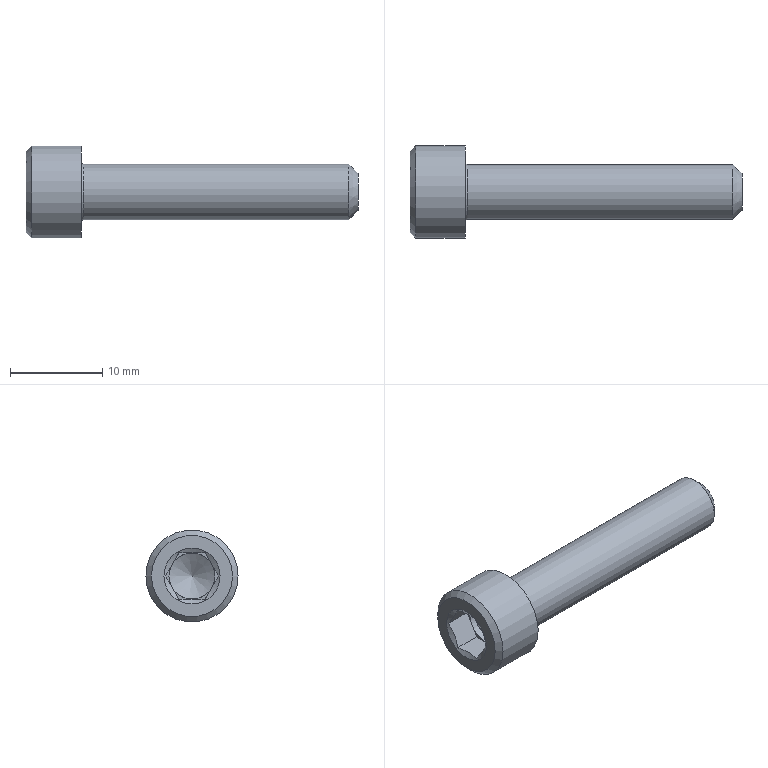Part | STEP file | Винт М6-6gx30 ГОСТ 11738-84 | 1 solid | 23 faces | box 36 x 10 x 10 mm | volume 1217 mm3 | plane 15 | cone 4 | cylinder 3 | torus 1 | commonest cylinder face diameters 5 x1 6 x1 10 x1
STEP:
#1=CARTESIAN_POINT('',(-6.,4.4,0.));
#2=VERTEX_POINT('',#1);
#3=CARTESIAN_POINT('',(-6.,0.,0.));
#4=DIRECTION('',(1.,0.,0.));
#5=DIRECTION('',(0.,1.,0.));
#6=AXIS2_PLACEMENT_3D('',#3,#4,#5);
#7=CIRCLE('',#6,4.4);
#8=EDGE_CURVE('',#2,#2,#7,.T.);
#9=ORIENTED_EDGE('',*,*,#8,.F.);
#10=EDGE_LOOP('',(#9));
#11=FACE_BOUND('',#10,.T.);
#12=CARTESIAN_POINT('',(-6.,3.05,0.));
#13=VERTEX_POINT('',#12);
#14=CARTESIAN_POINT('',(-6.,0.,0.));
#15=DIRECTION('',(1.,0.,0.));
#16=DIRECTION('',(0.,1.,0.));
#17=AXIS2_PLACEMENT_3D('',#14,#15,#16);
#18=CIRCLE('',#17,3.05);
#19=EDGE_CURVE('',#13,#13,#18,.T.);
#20=ORIENTED_EDGE('',*,*,#19,.T.);
#21=EDGE_LOOP('',(#20));
#22=FACE_BOUND('',#21,.T.);
#23=CARTESIAN_POINT('',(-6.,0.,0.));
#24=DIRECTION('',(-1.,0.,0.));
#25=DIRECTION('',(0.,1.,0.));
#26=AXIS2_PLACEMENT_3D('',#23,#24,#25);
#27=PLANE('',#26);
#28=ADVANCED_FACE('',(#11,#22),#27,.T.);
#29=CARTESIAN_POINT('',(-5.906,1.443,-2.5));
#30=VERTEX_POINT('',#29);
#31=CARTESIAN_POINT('',(-5.906,-1.443,-2.5));
#32=VERTEX_POINT('',#31);
#33=CARTESIAN_POINT('',(-5.906,1.443,-2.5));
#34=CARTESIAN_POINT('',(-5.9,1.424,-2.5));
#35=CARTESIAN_POINT('',(-5.89,1.389,-2.5));
#36=CARTESIAN_POINT('',(-5.88,1.351,-2.5));
#37=CARTESIAN_POINT('',(-5.867,1.304,-2.5));
#38=CARTESIAN_POINT('',(-5.848,1.232,-2.5));
#39=CARTESIAN_POINT('',(-5.827,1.146,-2.5));
#40=CARTESIAN_POINT('',(-5.803,1.043,-2.5));
#41=CARTESIAN_POINT('',(-5.774,0.909,-2.5));
#42=CARTESIAN_POINT('',(-5.75,0.7773,-2.5));
#43=CARTESIAN_POINT('',(-5.728,0.6356,-2.5));
#44=CARTESIAN_POINT('',(-5.711,0.5115,-2.5));
#45=CARTESIAN_POINT('',(-5.699,0.3892,-2.5));
#46=CARTESIAN_POINT('',(-5.692,0.2947,-2.5));
#47=CARTESIAN_POINT('',(-5.688,0.2222,-2.5));
#48=CARTESIAN_POINT('',(-5.684,0.1323,-2.5));
#49=CARTESIAN_POINT('',(-5.683,0.05578,-2.5));
#50=CARTESIAN_POINT('',(-5.682,-0.001577,-2.5));
#51=CARTESIAN_POINT('',(-5.683,-0.03169,-2.5));
#52=CARTESIAN_POINT('',(-5.683,-0.0738,-2.5));
#53=CARTESIAN_POINT('',(-5.684,-0.1276,-2.5));
#54=CARTESIAN_POINT('',(-5.687,-0.2055,-2.5));
#55=CARTESIAN_POINT('',(-5.692,-0.2839,-2.5));
#56=CARTESIAN_POINT('',(-5.696,-0.3444,-2.5));
#57=CARTESIAN_POINT('',(-5.7,-0.3959,-2.5));
#58=CARTESIAN_POINT('',(-5.705,-0.4472,-2.5));
#59=CARTESIAN_POINT('',(-5.713,-0.5148,-2.5));
#60=CARTESIAN_POINT('',(-5.722,-0.5907,-2.5));
#61=CARTESIAN_POINT('',(-5.73,-0.6507,-2.5));
#62=CARTESIAN_POINT('',(-5.738,-0.7005,-2.5));
#63=CARTESIAN_POINT('',(-5.746,-0.7498,-2.5));
#64=CARTESIAN_POINT('',(-5.757,-0.8136,-2.5));
#65=CARTESIAN_POINT('',(-5.77,-0.8864,-2.5));
#66=CARTESIAN_POINT('',(-5.785,-0.9583,-2.5));
#67=CARTESIAN_POINT('',(-5.8,-1.03,-2.5));
#68=CARTESIAN_POINT('',(-5.812,-1.084,-2.5));
#69=CARTESIAN_POINT('',(-5.823,-1.131,-2.5));
#70=CARTESIAN_POINT('',(-5.834,-1.177,-2.5));
#71=CARTESIAN_POINT('',(-5.85,-1.239,-2.5));
#72=CARTESIAN_POINT('',(-5.868,-1.307,-2.5));
#73=CARTESIAN_POINT('',(-5.882,-1.361,-2.5));
#74=CARTESIAN_POINT('',(-5.895,-1.406,-2.5));
#75=CARTESIAN_POINT('',(-5.902,-1.429,-2.5));
#76=CARTESIAN_POINT('',(-5.906,-1.443,-2.5));
#77=B_SPLINE_CURVE_WITH_KNOTS('',3,(#33,#34,#35,#36,#37,#38,#39,#40,#41,#42,#43,#44,#45,#46,#47,#48,#49,#50,#51,#52,#53,#54,#55,#56,#57,#58,#59,#60,#61,#62,#63,#64,#65,#66,#67,#68,#69,#70,#71,#72,#73,#74,#75,#76),.UNSPECIFIED.,.F.,.F.,(4,1,1,1,1,1,1,1,1,1,1,1,1,1,1,1,1,1,1,1,1,1,1,1,1,1,1,1,1,1,1,1,1,1,1,1,1,1,1,1,1,4),(0.,0.02097,0.03685,0.04095,0.07015,0.1134,0.1316,0.1778,0.2541,0.2686,0.3246,0.3823,0.3943,0.4217,0.4566,0.4863,0.5,0.5153,0.5171,0.5431,0.5703,0.5969,0.6234,0.6325,0.6498,0.6761,0.7022,0.7281,0.7381,0.7538,0.7792,0.8044,0.8294,0.8543,0.8789,0.8866,0.9033,0.9276,0.9518,0.9759,0.9843,1.),.UNSPECIFIED.);
#78=EDGE_CURVE('',#30,#32,#77,.T.);
#79=ORIENTED_EDGE('',*,*,#78,.T.);
#80=CARTESIAN_POINT('',(-3.,-1.443,-2.5));
#81=VERTEX_POINT('',#80);
#82=CARTESIAN_POINT('',(-3.,-1.443,-2.5));
#83=DIRECTION('',(-1.,0.,0.));
#84=VECTOR('',#83,1.);
#85=LINE('',#82,#84);
#86=EDGE_CURVE('',#81,#32,#85,.T.);
#87=ORIENTED_EDGE('',*,*,#86,.F.);
#88=CARTESIAN_POINT('',(-3.,0.,-2.5));
#89=VERTEX_POINT('',#88);
#90=CARTESIAN_POINT('',(-3.,0.,-2.5));
#91=DIRECTION('',(0.,-1.,0.));
#92=VECTOR('',#91,1.);
#93=LINE('',#90,#92);
#94=EDGE_CURVE('',#89,#81,#93,.T.);
#95=ORIENTED_EDGE('',*,*,#94,.F.);
#96=CARTESIAN_POINT('',(-3.,1.443,-2.5));
#97=VERTEX_POINT('',#96);
#98=CARTESIAN_POINT('',(-3.,1.443,-2.5));
#99=DIRECTION('',(0.,-1.,0.));
#100=VECTOR('',#99,1.);
#101=LINE('',#98,#100);
#102=EDGE_CURVE('',#97,#89,#101,.T.);
#103=ORIENTED_EDGE('',*,*,#102,.F.);
#104=CARTESIAN_POINT('',(-3.,1.443,-2.5));
#105=DIRECTION('',(-1.,0.,0.));
#106=VECTOR('',#105,1.);
#107=LINE('',#104,#106);
#108=EDGE_CURVE('',#97,#30,#107,.T.);
#109=ORIENTED_EDGE('',*,*,#108,.T.);
#110=EDGE_LOOP('',(#79,#87,#95,#103,#109));
#111=FACE_BOUND('',#110,.T.);
#112=CARTESIAN_POINT('',(-3.,1.443,-2.5));
#113=DIRECTION('',(0.,0.,-1.));
#114=DIRECTION('',(0.,-1.,0.));
#115=AXIS2_PLACEMENT_3D('',#112,#113,#114);
#116=PLANE('',#115);
#117=ADVANCED_FACE('',(#111),#116,.F.);
#118=CARTESIAN_POINT('',(-5.906,-2.887,0.));
#119=VERTEX_POINT('',#118);
#120=CARTESIAN_POINT('',(-5.906,-1.443,-2.5));
#121=CARTESIAN_POINT('',(-5.9,-1.453,-2.483));
#122=CARTESIAN_POINT('',(-5.889,-1.472,-2.45));
#123=CARTESIAN_POINT('',(-5.871,-1.505,-2.392));
#124=CARTESIAN_POINT('',(-5.848,-1.549,-2.317));
#125=CARTESIAN_POINT('',(-5.816,-1.614,-2.204));
#126=CARTESIAN_POINT('',(-5.777,-1.702,-2.052));
#127=CARTESIAN_POINT('',(-5.74,-1.803,-1.877));
#128=CARTESIAN_POINT('',(-5.713,-1.902,-1.705));
#129=CARTESIAN_POINT('',(-5.697,-1.984,-1.564));
#130=CARTESIAN_POINT('',(-5.688,-2.048,-1.453));
#131=CARTESIAN_POINT('',(-5.684,-2.099,-1.365));
#132=CARTESIAN_POINT('',(-5.683,-2.137,-1.298));
#133=CARTESIAN_POINT('',(-5.682,-2.166,-1.249));
#134=CARTESIAN_POINT('',(-5.683,-2.194,-1.201));
#135=CARTESIAN_POINT('',(-5.684,-2.228,-1.141));
#136=CARTESIAN_POINT('',(-5.687,-2.268,-1.072));
#137=CARTESIAN_POINT('',(-5.692,-2.307,-1.004));
#138=CARTESIAN_POINT('',(-5.697,-2.346,-0.9371));
#139=CARTESIAN_POINT('',(-5.704,-2.384,-0.8704));
#140=CARTESIAN_POINT('',(-5.713,-2.422,-0.8041));
#141=CARTESIAN_POINT('',(-5.722,-2.46,-0.7384));
#142=CARTESIAN_POINT('',(-5.733,-2.498,-0.6734));
#143=CARTESIAN_POINT('',(-5.744,-2.535,-0.609));
#144=CARTESIAN_POINT('',(-5.757,-2.572,-0.5454));
#145=CARTESIAN_POINT('',(-5.77,-2.608,-0.4824));
#146=CARTESIAN_POINT('',(-5.785,-2.644,-0.4201));
#147=CARTESIAN_POINT('',(-5.8,-2.68,-0.3584));
#148=CARTESIAN_POINT('',(-5.816,-2.715,-0.2974));
#149=CARTESIAN_POINT('',(-5.832,-2.75,-0.237));
#150=CARTESIAN_POINT('',(-5.85,-2.784,-0.1771));
#151=CARTESIAN_POINT('',(-5.868,-2.819,-0.1177));
#152=CARTESIAN_POINT('',(-5.886,-2.853,-0.05869));
#153=CARTESIAN_POINT('',(-5.899,-2.875,-0.01952));
#154=CARTESIAN_POINT('',(-5.906,-2.887,0.));
#155=B_SPLINE_CURVE_WITH_KNOTS('',3,(#120,#121,#122,#123,#124,#125,#126,#127,#128,#129,#130,#131,#132,#133,#134,#135,#136,#137,#138,#139,#140,#141,#142,#143,#144,#145,#146,#147,#148,#149,#150,#151,#152,#153,#154),.UNSPECIFIED.,.F.,.F.,(4,1,1,1,1,1,1,1,1,1,1,1,1,1,1,1,1,1,1,1,1,1,1,1,1,1,1,1,1,1,1,1,4),(0.,0.02097,0.04095,0.07015,0.1134,0.1778,0.2541,0.3246,0.3823,0.4217,0.4566,0.4863,0.5,0.5153,0.5431,0.5703,0.5969,0.6234,0.6498,0.6761,0.7022,0.7281,0.7538,0.7792,0.8044,0.8294,0.8543,0.8789,0.9033,0.9276,0.9518,0.9759,1.),.UNSPECIFIED.);
#156=EDGE_CURVE('',#32,#119,#155,.T.);
#157=ORIENTED_EDGE('',*,*,#156,.T.);
#158=CARTESIAN_POINT('',(-3.,-2.887,0.));
#159=VERTEX_POINT('',#158);
#160=CARTESIAN_POINT('',(-3.,-2.887,0.));
#161=DIRECTION('',(-1.,0.,0.));
#162=VECTOR('',#161,1.);
#163=LINE('',#160,#162);
#164=EDGE_CURVE('',#159,#119,#163,.T.);
#165=ORIENTED_EDGE('',*,*,#164,.F.);
#166=CARTESIAN_POINT('',(-3.,-2.165,-1.25));
#167=VERTEX_POINT('',#166);
#168=CARTESIAN_POINT('',(-3.,-2.165,-1.25));
#169=DIRECTION('',(0.,-0.5,0.866));
#170=VECTOR('',#169,1.);
#171=LINE('',#168,#170);
#172=EDGE_CURVE('',#167,#159,#171,.T.);
#173=ORIENTED_EDGE('',*,*,#172,.F.);
#174=CARTESIAN_POINT('',(-3.,-1.443,-2.5));
#175=DIRECTION('',(0.,-0.5,0.866));
#176=VECTOR('',#175,1.);
#177=LINE('',#174,#176);
#178=EDGE_CURVE('',#81,#167,#177,.T.);
#179=ORIENTED_EDGE('',*,*,#178,.F.);
#180=ORIENTED_EDGE('',*,*,#86,.T.);
#181=EDGE_LOOP('',(#157,#165,#173,#179,#180));
#182=FACE_BOUND('',#181,.T.);
#183=CARTESIAN_POINT('',(-3.,-1.443,-2.5));
#184=DIRECTION('',(0.,-0.866,-0.5));
#185=DIRECTION('',(0.,-0.5,0.866));
#186=AXIS2_PLACEMENT_3D('',#183,#184,#185);
#187=PLANE('',#186);
#188=ADVANCED_FACE('',(#182),#187,.F.);
#189=CARTESIAN_POINT('',(-5.906,-1.443,2.5));
#190=VERTEX_POINT('',#189);
#191=CARTESIAN_POINT('',(-5.906,-2.887,0.));
#192=CARTESIAN_POINT('',(-5.9,-2.877,0.01704));
#193=CARTESIAN_POINT('',(-5.889,-2.858,0.05036));
#194=CARTESIAN_POINT('',(-5.871,-2.825,0.1076));
#195=CARTESIAN_POINT('',(-5.848,-2.781,0.1832));
#196=CARTESIAN_POINT('',(-5.816,-2.716,0.2956));
#197=CARTESIAN_POINT('',(-5.777,-2.628,0.4476));
#198=CARTESIAN_POINT('',(-5.74,-2.527,0.6235));
#199=CARTESIAN_POINT('',(-5.713,-2.428,0.7948));
#200=CARTESIAN_POINT('',(-5.697,-2.346,0.936));
#201=CARTESIAN_POINT('',(-5.688,-2.282,1.047));
#202=CARTESIAN_POINT('',(-5.684,-2.231,1.135));
#203=CARTESIAN_POINT('',(-5.683,-2.193,1.202));
#204=CARTESIAN_POINT('',(-5.682,-2.164,1.251));
#205=CARTESIAN_POINT('',(-5.683,-2.137,1.299));
#206=CARTESIAN_POINT('',(-5.684,-2.102,1.359));
#207=CARTESIAN_POINT('',(-5.687,-2.062,1.428));
#208=CARTESIAN_POINT('',(-5.692,-2.023,1.496));
#209=CARTESIAN_POINT('',(-5.697,-1.984,1.563));
#210=CARTESIAN_POINT('',(-5.704,-1.946,1.63));
#211=CARTESIAN_POINT('',(-5.713,-1.908,1.696));
#212=CARTESIAN_POINT('',(-5.722,-1.87,1.762));
#213=CARTESIAN_POINT('',(-5.733,-1.832,1.827));
#214=CARTESIAN_POINT('',(-5.744,-1.795,1.891));
#215=CARTESIAN_POINT('',(-5.757,-1.758,1.955));
#216=CARTESIAN_POINT('',(-5.77,-1.722,2.018));
#217=CARTESIAN_POINT('',(-5.785,-1.686,2.08));
#218=CARTESIAN_POINT('',(-5.8,-1.65,2.142));
#219=CARTESIAN_POINT('',(-5.816,-1.615,2.203));
#220=CARTESIAN_POINT('',(-5.832,-1.58,2.263));
#221=CARTESIAN_POINT('',(-5.85,-1.546,2.323));
#222=CARTESIAN_POINT('',(-5.868,-1.511,2.382));
#223=CARTESIAN_POINT('',(-5.886,-1.477,2.441));
#224=CARTESIAN_POINT('',(-5.899,-1.455,2.48));
#225=CARTESIAN_POINT('',(-5.906,-1.443,2.5));
#226=B_SPLINE_CURVE_WITH_KNOTS('',3,(#191,#192,#193,#194,#195,#196,#197,#198,#199,#200,#201,#202,#203,#204,#205,#206,#207,#208,#209,#210,#211,#212,#213,#214,#215,#216,#217,#218,#219,#220,#221,#222,#223,#224,#225),.UNSPECIFIED.,.F.,.F.,(4,1,1,1,1,1,1,1,1,1,1,1,1,1,1,1,1,1,1,1,1,1,1,1,1,1,1,1,1,1,1,1,4),(0.,0.02097,0.04095,0.07015,0.1134,0.1778,0.2541,0.3246,0.3823,0.4217,0.4566,0.4863,0.5,0.5153,0.5431,0.5703,0.5969,0.6234,0.6498,0.6761,0.7022,0.7281,0.7538,0.7792,0.8044,0.8294,0.8543,0.8789,0.9033,0.9276,0.9518,0.9759,1.),.UNSPECIFIED.);
#227=EDGE_CURVE('',#119,#190,#226,.T.);
#228=ORIENTED_EDGE('',*,*,#227,.T.);
#229=CARTESIAN_POINT('',(-3.,-1.443,2.5));
#230=VERTEX_POINT('',#229);
#231=CARTESIAN_POINT('',(-3.,-1.443,2.5));
#232=DIRECTION('',(-1.,0.,0.));
#233=VECTOR('',#232,1.);
#234=LINE('',#231,#233);
#235=EDGE_CURVE('',#230,#190,#234,.T.);
#236=ORIENTED_EDGE('',*,*,#235,.F.);
#237=CARTESIAN_POINT('',(-3.,-2.165,1.25));
#238=VERTEX_POINT('',#237);
#239=CARTESIAN_POINT('',(-3.,-2.165,1.25));
#240=DIRECTION('',(0.,0.5,0.866));
#241=VECTOR('',#240,1.);
#242=LINE('',#239,#241);
#243=EDGE_CURVE('',#238,#230,#242,.T.);
#244=ORIENTED_EDGE('',*,*,#243,.F.);
#245=CARTESIAN_POINT('',(-3.,-2.887,0.));
#246=DIRECTION('',(0.,0.5,0.866));
#247=VECTOR('',#246,1.);
#248=LINE('',#245,#247);
#249=EDGE_CURVE('',#159,#238,#248,.T.);
#250=ORIENTED_EDGE('',*,*,#249,.F.);
#251=ORIENTED_EDGE('',*,*,#164,.T.);
#252=EDGE_LOOP('',(#228,#236,#244,#250,#251));
#253=FACE_BOUND('',#252,.T.);
#254=CARTESIAN_POINT('',(-3.,-2.887,0.));
#255=DIRECTION('',(0.,-0.866,0.5));
#256=DIRECTION('',(0.,0.5,0.866));
#257=AXIS2_PLACEMENT_3D('',#254,#255,#256);
#258=PLANE('',#257);
#259=ADVANCED_FACE('',(#253),#258,.F.);
#260=CARTESIAN_POINT('',(-5.906,1.443,2.5));
#261=VERTEX_POINT('',#260);
#262=CARTESIAN_POINT('',(-5.906,-1.443,2.5));
#263=CARTESIAN_POINT('',(-5.9,-1.424,2.5));
#264=CARTESIAN_POINT('',(-5.89,-1.389,2.5));
#265=CARTESIAN_POINT('',(-5.88,-1.351,2.5));
#266=CARTESIAN_POINT('',(-5.867,-1.304,2.5));
#267=CARTESIAN_POINT('',(-5.848,-1.232,2.5));
#268=CARTESIAN_POINT('',(-5.827,-1.146,2.5));
#269=CARTESIAN_POINT('',(-5.803,-1.043,2.5));
#270=CARTESIAN_POINT('',(-5.774,-0.909,2.5));
#271=CARTESIAN_POINT('',(-5.75,-0.7773,2.5));
#272=CARTESIAN_POINT('',(-5.728,-0.6356,2.5));
#273=CARTESIAN_POINT('',(-5.711,-0.5115,2.5));
#274=CARTESIAN_POINT('',(-5.699,-0.3892,2.5));
#275=CARTESIAN_POINT('',(-5.692,-0.2947,2.5));
#276=CARTESIAN_POINT('',(-5.688,-0.2222,2.5));
#277=CARTESIAN_POINT('',(-5.684,-0.1323,2.5));
#278=CARTESIAN_POINT('',(-5.683,-0.05578,2.5));
#279=CARTESIAN_POINT('',(-5.682,0.001577,2.5));
#280=CARTESIAN_POINT('',(-5.683,0.03169,2.5));
#281=CARTESIAN_POINT('',(-5.683,0.0738,2.5));
#282=CARTESIAN_POINT('',(-5.684,0.1276,2.5));
#283=CARTESIAN_POINT('',(-5.687,0.2055,2.5));
#284=CARTESIAN_POINT('',(-5.692,0.2839,2.5));
#285=CARTESIAN_POINT('',(-5.696,0.3444,2.5));
#286=CARTESIAN_POINT('',(-5.7,0.3959,2.5));
#287=CARTESIAN_POINT('',(-5.705,0.4472,2.5));
#288=CARTESIAN_POINT('',(-5.713,0.5148,2.5));
#289=CARTESIAN_POINT('',(-5.722,0.5907,2.5));
#290=CARTESIAN_POINT('',(-5.73,0.6507,2.5));
#291=CARTESIAN_POINT('',(-5.738,0.7005,2.5));
#292=CARTESIAN_POINT('',(-5.746,0.7498,2.5));
#293=CARTESIAN_POINT('',(-5.757,0.8136,2.5));
#294=CARTESIAN_POINT('',(-5.77,0.8864,2.5));
#295=CARTESIAN_POINT('',(-5.785,0.9583,2.5));
#296=CARTESIAN_POINT('',(-5.8,1.03,2.5));
#297=CARTESIAN_POINT('',(-5.812,1.084,2.5));
#298=CARTESIAN_POINT('',(-5.823,1.131,2.5));
#299=CARTESIAN_POINT('',(-5.834,1.177,2.5));
#300=CARTESIAN_POINT('',(-5.85,1.239,2.5));
#301=CARTESIAN_POINT('',(-5.868,1.307,2.5));
#302=CARTESIAN_POINT('',(-5.882,1.361,2.5));
#303=CARTESIAN_POINT('',(-5.895,1.406,2.5));
#304=CARTESIAN_POINT('',(-5.902,1.429,2.5));
#305=CARTESIAN_POINT('',(-5.906,1.443,2.5));
#306=B_SPLINE_CURVE_WITH_KNOTS('',3,(#262,#263,#264,#265,#266,#267,#268,#269,#270,#271,#272,#273,#274,#275,#276,#277,#278,#279,#280,#281,#282,#283,#284,#285,#286,#287,#288,#289,#290,#291,#292,#293,#294,#295,#296,#297,#298,#299,#300,#301,#302,#303,#304,#305),.UNSPECIFIED.,.F.,.F.,(4,1,1,1,1,1,1,1,1,1,1,1,1,1,1,1,1,1,1,1,1,1,1,1,1,1,1,1,1,1,1,1,1,1,1,1,1,1,1,1,1,4),(0.,0.02097,0.03685,0.04095,0.07015,0.1134,0.1316,0.1778,0.2541,0.2686,0.3246,0.3823,0.3943,0.4217,0.4566,0.4863,0.5,0.5153,0.5171,0.5431,0.5703,0.5969,0.6234,0.6325,0.6498,0.6761,0.7022,0.7281,0.7381,0.7538,0.7792,0.8044,0.8294,0.8543,0.8789,0.8866,0.9033,0.9276,0.9518,0.9759,0.9843,1.),.UNSPECIFIED.);
#307=EDGE_CURVE('',#190,#261,#306,.T.);
#308=ORIENTED_EDGE('',*,*,#307,.T.);
#309=CARTESIAN_POINT('',(-3.,1.443,2.5));
#310=VERTEX_POINT('',#309);
#311=CARTESIAN_POINT('',(-3.,1.443,2.5));
#312=DIRECTION('',(-1.,0.,0.));
#313=VECTOR('',#312,1.);
#314=LINE('',#311,#313);
#315=EDGE_CURVE('',#310,#261,#314,.T.);
#316=ORIENTED_EDGE('',*,*,#315,.F.);
#317=CARTESIAN_POINT('',(-3.,0.,2.5));
#318=VERTEX_POINT('',#317);
#319=CARTESIAN_POINT('',(-3.,0.,2.5));
#320=DIRECTION('',(0.,1.,0.));
#321=VECTOR('',#320,1.);
#322=LINE('',#319,#321);
#323=EDGE_CURVE('',#318,#310,#322,.T.);
#324=ORIENTED_EDGE('',*,*,#323,.F.);
#325=CARTESIAN_POINT('',(-3.,-1.443,2.5));
#326=DIRECTION('',(0.,1.,0.));
#327=VECTOR('',#326,1.);
#328=LINE('',#325,#327);
#329=EDGE_CURVE('',#230,#318,#328,.T.);
#330=ORIENTED_EDGE('',*,*,#329,.F.);
#331=ORIENTED_EDGE('',*,*,#235,.T.);
#332=EDGE_LOOP('',(#308,#316,#324,#330,#331));
#333=FACE_BOUND('',#332,.T.);
#334=CARTESIAN_POINT('',(-3.,-1.443,2.5));
#335=DIRECTION('',(0.,0.,1.));
#336=DIRECTION('',(0.,1.,0.));
#337=AXIS2_PLACEMENT_3D('',#334,#335,#336);
#338=PLANE('',#337);
#339=ADVANCED_FACE('',(#333),#338,.F.);
#340=CARTESIAN_POINT('',(-5.906,2.887,0.));
#341=VERTEX_POINT('',#340);
#342=CARTESIAN_POINT('',(-5.906,2.887,0.));
#343=CARTESIAN_POINT('',(-5.9,2.877,-0.01704));
#344=CARTESIAN_POINT('',(-5.889,2.858,-0.05036));
#345=CARTESIAN_POINT('',(-5.871,2.825,-0.1076));
#346=CARTESIAN_POINT('',(-5.848,2.781,-0.1832));
#347=CARTESIAN_POINT('',(-5.816,2.716,-0.2956));
#348=CARTESIAN_POINT('',(-5.777,2.628,-0.4476));
#349=CARTESIAN_POINT('',(-5.74,2.527,-0.6235));
#350=CARTESIAN_POINT('',(-5.713,2.428,-0.7948));
#351=CARTESIAN_POINT('',(-5.697,2.346,-0.936));
#352=CARTESIAN_POINT('',(-5.688,2.282,-1.047));
#353=CARTESIAN_POINT('',(-5.684,2.231,-1.135));
#354=CARTESIAN_POINT('',(-5.683,2.193,-1.202));
#355=CARTESIAN_POINT('',(-5.682,2.164,-1.251));
#356=CARTESIAN_POINT('',(-5.683,2.137,-1.299));
#357=CARTESIAN_POINT('',(-5.684,2.102,-1.359));
#358=CARTESIAN_POINT('',(-5.687,2.062,-1.428));
#359=CARTESIAN_POINT('',(-5.692,2.023,-1.496));
#360=CARTESIAN_POINT('',(-5.697,1.984,-1.563));
#361=CARTESIAN_POINT('',(-5.704,1.946,-1.63));
#362=CARTESIAN_POINT('',(-5.713,1.908,-1.696));
#363=CARTESIAN_POINT('',(-5.722,1.87,-1.762));
#364=CARTESIAN_POINT('',(-5.733,1.832,-1.827));
#365=CARTESIAN_POINT('',(-5.744,1.795,-1.891));
#366=CARTESIAN_POINT('',(-5.757,1.758,-1.955));
#367=CARTESIAN_POINT('',(-5.77,1.722,-2.018));
#368=CARTESIAN_POINT('',(-5.785,1.686,-2.08));
#369=CARTESIAN_POINT('',(-5.8,1.65,-2.142));
#370=CARTESIAN_POINT('',(-5.816,1.615,-2.203));
#371=CARTESIAN_POINT('',(-5.832,1.58,-2.263));
#372=CARTESIAN_POINT('',(-5.85,1.546,-2.323));
#373=CARTESIAN_POINT('',(-5.868,1.511,-2.382));
#374=CARTESIAN_POINT('',(-5.886,1.477,-2.441));
#375=CARTESIAN_POINT('',(-5.899,1.455,-2.48));
#376=CARTESIAN_POINT('',(-5.906,1.443,-2.5));
#377=B_SPLINE_CURVE_WITH_KNOTS('',3,(#342,#343,#344,#345,#346,#347,#348,#349,#350,#351,#352,#353,#354,#355,#356,#357,#358,#359,#360,#361,#362,#363,#364,#365,#366,#367,#368,#369,#370,#371,#372,#373,#374,#375,#376),.UNSPECIFIED.,.F.,.F.,(4,1,1,1,1,1,1,1,1,1,1,1,1,1,1,1,1,1,1,1,1,1,1,1,1,1,1,1,1,1,1,1,4),(0.,0.02097,0.04095,0.07015,0.1134,0.1778,0.2541,0.3246,0.3823,0.4217,0.4566,0.4863,0.5,0.5153,0.5431,0.5703,0.5969,0.6234,0.6498,0.6761,0.7022,0.7281,0.7538,0.7792,0.8044,0.8294,0.8543,0.8789,0.9033,0.9276,0.9518,0.9759,1.),.UNSPECIFIED.);
#378=EDGE_CURVE('',#341,#30,#377,.T.);
#379=ORIENTED_EDGE('',*,*,#378,.T.);
#380=ORIENTED_EDGE('',*,*,#108,.F.);
#381=CARTESIAN_POINT('',(-3.,2.165,-1.25));
#382=VERTEX_POINT('',#381);
#383=CARTESIAN_POINT('',(-3.,2.165,-1.25));
#384=DIRECTION('',(0.,-0.5,-0.866));
#385=VECTOR('',#384,1.);
#386=LINE('',#383,#385);
#387=EDGE_CURVE('',#382,#97,#386,.T.);
#388=ORIENTED_EDGE('',*,*,#387,.F.);
#389=CARTESIAN_POINT('',(-3.,2.887,0.));
#390=VERTEX_POINT('',#389);
#391=CARTESIAN_POINT('',(-3.,2.887,0.));
#392=DIRECTION('',(0.,-0.5,-0.866));
#393=VECTOR('',#392,1.);
#394=LINE('',#391,#393);
#395=EDGE_CURVE('',#390,#382,#394,.T.);
#396=ORIENTED_EDGE('',*,*,#395,.F.);
#397=CARTESIAN_POINT('',(-3.,2.887,0.));
#398=DIRECTION('',(-1.,0.,0.));
#399=VECTOR('',#398,1.);
#400=LINE('',#397,#399);
#401=EDGE_CURVE('',#390,#341,#400,.T.);
#402=ORIENTED_EDGE('',*,*,#401,.T.);
#403=EDGE_LOOP('',(#379,#380,#388,#396,#402));
#404=FACE_BOUND('',#403,.T.);
#405=CARTESIAN_POINT('',(-3.,2.887,0.));
#406=DIRECTION('',(0.,0.866,-0.5));
#407=DIRECTION('',(0.,-0.5,-0.866));
#408=AXIS2_PLACEMENT_3D('',#405,#406,#407);
#409=PLANE('',#408);
#410=ADVANCED_FACE('',(#404),#409,.F.);
#411=CARTESIAN_POINT('',(-5.906,1.443,2.5));
#412=CARTESIAN_POINT('',(-5.9,1.453,2.483));
#413=CARTESIAN_POINT('',(-5.889,1.472,2.45));
#414=CARTESIAN_POINT('',(-5.871,1.505,2.392));
#415=CARTESIAN_POINT('',(-5.848,1.549,2.317));
#416=CARTESIAN_POINT('',(-5.816,1.614,2.204));
#417=CARTESIAN_POINT('',(-5.777,1.702,2.052));
#418=CARTESIAN_POINT('',(-5.74,1.803,1.877));
#419=CARTESIAN_POINT('',(-5.713,1.902,1.705));
#420=CARTESIAN_POINT('',(-5.697,1.984,1.564));
#421=CARTESIAN_POINT('',(-5.688,2.048,1.453));
#422=CARTESIAN_POINT('',(-5.684,2.099,1.365));
#423=CARTESIAN_POINT('',(-5.683,2.137,1.298));
#424=CARTESIAN_POINT('',(-5.682,2.166,1.249));
#425=CARTESIAN_POINT('',(-5.683,2.194,1.201));
#426=CARTESIAN_POINT('',(-5.684,2.228,1.141));
#427=CARTESIAN_POINT('',(-5.687,2.268,1.072));
#428=CARTESIAN_POINT('',(-5.692,2.307,1.004));
#429=CARTESIAN_POINT('',(-5.697,2.346,0.9371));
#430=CARTESIAN_POINT('',(-5.704,2.384,0.8704));
#431=CARTESIAN_POINT('',(-5.713,2.422,0.8041));
#432=CARTESIAN_POINT('',(-5.722,2.46,0.7384));
#433=CARTESIAN_POINT('',(-5.733,2.498,0.6734));
#434=CARTESIAN_POINT('',(-5.744,2.535,0.609));
#435=CARTESIAN_POINT('',(-5.757,2.572,0.5454));
#436=CARTESIAN_POINT('',(-5.77,2.608,0.4824));
#437=CARTESIAN_POINT('',(-5.785,2.644,0.4201));
#438=CARTESIAN_POINT('',(-5.8,2.68,0.3584));
#439=CARTESIAN_POINT('',(-5.816,2.715,0.2974));
#440=CARTESIAN_POINT('',(-5.832,2.75,0.237));
#441=CARTESIAN_POINT('',(-5.85,2.784,0.1771));
#442=CARTESIAN_POINT('',(-5.868,2.819,0.1177));
#443=CARTESIAN_POINT('',(-5.886,2.853,0.05869));
#444=CARTESIAN_POINT('',(-5.899,2.875,0.01952));
#445=CARTESIAN_POINT('',(-5.906,2.887,0.));
#446=B_SPLINE_CURVE_WITH_KNOTS('',3,(#411,#412,#413,#414,#415,#416,#417,#418,#419,#420,#421,#422,#423,#424,#425,#426,#427,#428,#429,#430,#431,#432,#433,#434,#435,#436,#437,#438,#439,#440,#441,#442,#443,#444,#445),.UNSPECIFIED.,.F.,.F.,(4,1,1,1,1,1,1,1,1,1,1,1,1,1,1,1,1,1,1,1,1,1,1,1,1,1,1,1,1,1,1,1,4),(0.,0.02097,0.04095,0.07015,0.1134,0.1778,0.2541,0.3246,0.3823,0.4217,0.4566,0.4863,0.5,0.5153,0.5431,0.5703,0.5969,0.6234,0.6498,0.6761,0.7022,0.7281,0.7538,0.7792,0.8044,0.8294,0.8543,0.8789,0.9033,0.9276,0.9518,0.9759,1.),.UNSPECIFIED.);
#447=EDGE_CURVE('',#261,#341,#446,.T.);
#448=ORIENTED_EDGE('',*,*,#447,.T.);
#449=ORIENTED_EDGE('',*,*,#401,.F.);
#450=CARTESIAN_POINT('',(-3.,2.165,1.25));
#451=VERTEX_POINT('',#450);
#452=CARTESIAN_POINT('',(-3.,2.165,1.25));
#453=DIRECTION('',(0.,0.5,-0.866));
#454=VECTOR('',#453,1.);
#455=LINE('',#452,#454);
#456=EDGE_CURVE('',#451,#390,#455,.T.);
#457=ORIENTED_EDGE('',*,*,#456,.F.);
#458=CARTESIAN_POINT('',(-3.,1.443,2.5));
#459=DIRECTION('',(0.,0.5,-0.866));
#460=VECTOR('',#459,1.);
#461=LINE('',#458,#460);
#462=EDGE_CURVE('',#310,#451,#461,.T.);
#463=ORIENTED_EDGE('',*,*,#462,.F.);
#464=ORIENTED_EDGE('',*,*,#315,.T.);
#465=EDGE_LOOP('',(#448,#449,#457,#463,#464));
#466=FACE_BOUND('',#465,.T.);
#467=CARTESIAN_POINT('',(-3.,1.443,2.5));
#468=DIRECTION('',(0.,0.866,0.5));
#469=DIRECTION('',(0.,0.5,-0.866));
#470=AXIS2_PLACEMENT_3D('',#467,#468,#469);
#471=PLANE('',#470);
#472=ADVANCED_FACE('',(#466),#471,.F.);
#473=ORIENTED_EDGE('',*,*,#447,.F.);
#474=ORIENTED_EDGE('',*,*,#307,.F.);
#475=ORIENTED_EDGE('',*,*,#227,.F.);
#476=ORIENTED_EDGE('',*,*,#156,.F.);
#477=ORIENTED_EDGE('',*,*,#78,.F.);
#478=ORIENTED_EDGE('',*,*,#378,.F.);
#479=EDGE_LOOP('',(#473,#474,#475,#476,#477,#478));
#480=FACE_BOUND('',#479,.T.);
#481=ORIENTED_EDGE('',*,*,#19,.F.);
#482=EDGE_LOOP('',(#481));
#483=FACE_OUTER_BOUND('',#482,.T.);
#484=CARTESIAN_POINT('',(-5.841,0.,0.));
#485=DIRECTION('',(-1.,0.,0.));
#486=DIRECTION('',(0.,-1.,0.));
#487=AXIS2_PLACEMENT_3D('',#484,#485,#486);
#488=CONICAL_SURFACE('',#487,2.775,1.047);
#489=ADVANCED_FACE('',(#480,#483),#488,.F.);
#490=CARTESIAN_POINT('',(-5.4,5.,0.));
#491=VERTEX_POINT('',#490);
#492=CARTESIAN_POINT('',(-5.4,0.,0.));
#493=DIRECTION('',(1.,0.,0.));
#494=DIRECTION('',(0.,1.,0.));
#495=AXIS2_PLACEMENT_3D('',#492,#493,#494);
#496=CIRCLE('',#495,5.);
#497=EDGE_CURVE('',#491,#491,#496,.T.);
#498=ORIENTED_EDGE('',*,*,#497,.F.);
#499=EDGE_LOOP('',(#498));
#500=FACE_OUTER_BOUND('',#499,.T.);
#501=ORIENTED_EDGE('',*,*,#8,.T.);
#502=EDGE_LOOP('',(#501));
#503=FACE_OUTER_BOUND('',#502,.T.);
#504=CARTESIAN_POINT('',(-5.7,0.,0.));
#505=DIRECTION('',(1.,0.,0.));
#506=DIRECTION('',(0.,1.,0.));
#507=AXIS2_PLACEMENT_3D('',#504,#505,#506);
#508=CONICAL_SURFACE('',#507,4.7,0.7854);
#509=ADVANCED_FACE('',(#500,#503),#508,.T.);
#510=CARTESIAN_POINT('',(-3.,0.,0.));
#511=DIRECTION('',(1.,0.,0.));
#512=DIRECTION('',(0.,-0.866,-0.5));
#513=AXIS2_PLACEMENT_3D('',#510,#511,#512);
#514=CIRCLE('',#513,2.5);
#515=EDGE_CURVE('',#167,#89,#514,.T.);
#516=ORIENTED_EDGE('',*,*,#515,.T.);
#517=ORIENTED_EDGE('',*,*,#94,.T.);
#518=ORIENTED_EDGE('',*,*,#178,.T.);
#519=EDGE_LOOP('',(#516,#517,#518));
#520=FACE_BOUND('',#519,.T.);
#521=CARTESIAN_POINT('',(-3.,0.,0.));
#522=DIRECTION('',(-1.,0.,0.));
#523=DIRECTION('',(0.,0.,-1.));
#524=AXIS2_PLACEMENT_3D('',#521,#522,#523);
#525=PLANE('',#524);
#526=ADVANCED_FACE('',(#520),#525,.T.);
#527=CARTESIAN_POINT('',(-3.,0.,0.));
#528=DIRECTION('',(1.,0.,0.));
#529=DIRECTION('',(0.,0.,-1.));
#530=AXIS2_PLACEMENT_3D('',#527,#528,#529);
#531=CIRCLE('',#530,2.5);
#532=EDGE_CURVE('',#89,#382,#531,.T.);
#533=ORIENTED_EDGE('',*,*,#532,.T.);
#534=ORIENTED_EDGE('',*,*,#387,.T.);
#535=ORIENTED_EDGE('',*,*,#102,.T.);
#536=EDGE_LOOP('',(#533,#534,#535));
#537=FACE_BOUND('',#536,.T.);
#538=CARTESIAN_POINT('',(-3.,0.,0.));
#539=DIRECTION('',(-1.,0.,0.));
#540=DIRECTION('',(0.,0.,-1.));
#541=AXIS2_PLACEMENT_3D('',#538,#539,#540);
#542=PLANE('',#541);
#543=ADVANCED_FACE('',(#537),#542,.T.);
#544=CARTESIAN_POINT('',(-3.,0.,0.));
#545=DIRECTION('',(1.,0.,0.));
#546=DIRECTION('',(0.,-0.866,0.5));
#547=AXIS2_PLACEMENT_3D('',#544,#545,#546);
#548=CIRCLE('',#547,2.5);
#549=EDGE_CURVE('',#238,#167,#548,.T.);
#550=ORIENTED_EDGE('',*,*,#549,.T.);
#551=ORIENTED_EDGE('',*,*,#172,.T.);
#552=ORIENTED_EDGE('',*,*,#249,.T.);
#553=EDGE_LOOP('',(#550,#551,#552));
#554=FACE_BOUND('',#553,.T.);
#555=CARTESIAN_POINT('',(-3.,0.,0.));
#556=DIRECTION('',(-1.,0.,0.));
#557=DIRECTION('',(0.,0.,-1.));
#558=AXIS2_PLACEMENT_3D('',#555,#556,#557);
#559=PLANE('',#558);
#560=ADVANCED_FACE('',(#554),#559,.T.);
#561=CARTESIAN_POINT('',(-3.,0.,0.));
#562=DIRECTION('',(1.,0.,0.));
#563=DIRECTION('',(0.,0.,1.));
#564=AXIS2_PLACEMENT_3D('',#561,#562,#563);
#565=CIRCLE('',#564,2.5);
#566=EDGE_CURVE('',#318,#238,#565,.T.);
#567=ORIENTED_EDGE('',*,*,#566,.T.);
#568=ORIENTED_EDGE('',*,*,#243,.T.);
#569=ORIENTED_EDGE('',*,*,#329,.T.);
#570=EDGE_LOOP('',(#567,#568,#569));
#571=FACE_BOUND('',#570,.T.);
#572=CARTESIAN_POINT('',(-3.,0.,0.));
#573=DIRECTION('',(-1.,0.,0.));
#574=DIRECTION('',(0.,0.,-1.));
#575=AXIS2_PLACEMENT_3D('',#572,#573,#574);
#576=PLANE('',#575);
#577=ADVANCED_FACE('',(#571),#576,.T.);
#578=CARTESIAN_POINT('',(-3.,0.,0.));
#579=DIRECTION('',(1.,0.,0.));
#580=DIRECTION('',(0.,0.866,0.5));
#581=AXIS2_PLACEMENT_3D('',#578,#579,#580);
#582=CIRCLE('',#581,2.5);
#583=EDGE_CURVE('',#451,#318,#582,.T.);
#584=ORIENTED_EDGE('',*,*,#583,.T.);
#585=ORIENTED_EDGE('',*,*,#323,.T.);
#586=ORIENTED_EDGE('',*,*,#462,.T.);
#587=EDGE_LOOP('',(#584,#585,#586));
#588=FACE_BOUND('',#587,.T.);
#589=CARTESIAN_POINT('',(-3.,0.,0.));
#590=DIRECTION('',(-1.,0.,0.));
#591=DIRECTION('',(0.,0.,-1.));
#592=AXIS2_PLACEMENT_3D('',#589,#590,#591);
#593=PLANE('',#592);
#594=ADVANCED_FACE('',(#588),#593,.T.);
#595=CARTESIAN_POINT('',(-3.,2.5,0.));
#596=VERTEX_POINT('',#595);
#597=CARTESIAN_POINT('',(-3.,0.,0.));
#598=DIRECTION('',(1.,0.,0.));
#599=DIRECTION('',(0.,1.,0.));
#600=AXIS2_PLACEMENT_3D('',#597,#598,#599);
#601=CIRCLE('',#600,2.5);
#602=EDGE_CURVE('',#596,#451,#601,.T.);
#603=ORIENTED_EDGE('',*,*,#602,.T.);
#604=ORIENTED_EDGE('',*,*,#456,.T.);
#605=ORIENTED_EDGE('',*,*,#395,.T.);
#606=CARTESIAN_POINT('',(-3.,0.,0.));
#607=DIRECTION('',(1.,0.,0.));
#608=DIRECTION('',(0.,0.866,-0.5));
#609=AXIS2_PLACEMENT_3D('',#606,#607,#608);
#610=CIRCLE('',#609,2.5);
#611=EDGE_CURVE('',#382,#596,#610,.T.);
#612=ORIENTED_EDGE('',*,*,#611,.T.);
#613=EDGE_LOOP('',(#603,#604,#605,#612));
#614=FACE_BOUND('',#613,.T.);
#615=CARTESIAN_POINT('',(-3.,0.,0.));
#616=DIRECTION('',(-1.,0.,0.));
#617=DIRECTION('',(0.,0.,-1.));
#618=AXIS2_PLACEMENT_3D('',#615,#616,#617);
#619=PLANE('',#618);
#620=ADVANCED_FACE('',(#614),#619,.T.);
#621=CARTESIAN_POINT('',(0.,5.,0.));
#622=VERTEX_POINT('',#621);
#623=CARTESIAN_POINT('',(0.,0.,0.));
#624=DIRECTION('',(1.,0.,0.));
#625=DIRECTION('',(0.,1.,0.));
#626=AXIS2_PLACEMENT_3D('',#623,#624,#625);
#627=CIRCLE('',#626,5.);
#628=EDGE_CURVE('',#622,#622,#627,.T.);
#629=ORIENTED_EDGE('',*,*,#628,.F.);
#630=EDGE_LOOP('',(#629));
#631=FACE_OUTER_BOUND('',#630,.T.);
#632=ORIENTED_EDGE('',*,*,#497,.T.);
#633=EDGE_LOOP('',(#632));
#634=FACE_OUTER_BOUND('',#633,.T.);
#635=CARTESIAN_POINT('',(-6.,0.,0.));
#636=DIRECTION('',(1.,0.,0.));
#637=DIRECTION('',(0.,1.,0.));
#638=AXIS2_PLACEMENT_3D('',#635,#636,#637);
#639=CYLINDRICAL_SURFACE('',#638,5.);
#640=ADVANCED_FACE('',(#631,#634),#639,.T.);
#641=CARTESIAN_POINT('',(-2.3,2.5,0.));
#642=VERTEX_POINT('',#641);
#643=CARTESIAN_POINT('',(-2.3,0.,0.));
#644=DIRECTION('',(1.,0.,0.));
#645=DIRECTION('',(0.,1.,0.));
#646=AXIS2_PLACEMENT_3D('',#643,#644,#645);
#647=CIRCLE('',#646,2.5);
#648=EDGE_CURVE('',#642,#642,#647,.T.);
#649=ORIENTED_EDGE('',*,*,#648,.T.);
#650=EDGE_LOOP('',(#649));
#651=FACE_OUTER_BOUND('',#650,.T.);
#652=ORIENTED_EDGE('',*,*,#611,.F.);
#653=ORIENTED_EDGE('',*,*,#532,.F.);
#654=ORIENTED_EDGE('',*,*,#515,.F.);
#655=ORIENTED_EDGE('',*,*,#549,.F.);
#656=ORIENTED_EDGE('',*,*,#566,.F.);
#657=ORIENTED_EDGE('',*,*,#583,.F.);
#658=ORIENTED_EDGE('',*,*,#602,.F.);
#659=EDGE_LOOP('',(#652,#653,#654,#655,#656,#657,#658));
#660=FACE_BOUND('',#659,.T.);
#661=CARTESIAN_POINT('',(-6.,0.,0.));
#662=DIRECTION('',(1.,0.,0.));
#663=DIRECTION('',(0.,1.,0.));
#664=AXIS2_PLACEMENT_3D('',#661,#662,#663);
#665=CYLINDRICAL_SURFACE('',#664,2.5);
#666=ADVANCED_FACE('',(#651,#660),#665,.F.);
#667=ORIENTED_EDGE('',*,*,#628,.T.);
#668=EDGE_LOOP('',(#667));
#669=FACE_BOUND('',#668,.T.);
#670=CARTESIAN_POINT('',(0.,0.,-3.25));
#671=VERTEX_POINT('',#670);
#672=CARTESIAN_POINT('',(0.,0.,0.));
#673=DIRECTION('',(-1.,0.,0.));
#674=DIRECTION('',(0.,0.,-1.));
#675=AXIS2_PLACEMENT_3D('',#672,#673,#674);
#676=CIRCLE('',#675,3.25);
#677=EDGE_CURVE('',#671,#671,#676,.T.);
#678=ORIENTED_EDGE('',*,*,#677,.T.);
#679=EDGE_LOOP('',(#678));
#680=FACE_BOUND('',#679,.T.);
#681=CARTESIAN_POINT('',(0.,0.,0.));
#682=DIRECTION('',(1.,0.,0.));
#683=DIRECTION('',(0.,1.,0.));
#684=AXIS2_PLACEMENT_3D('',#681,#682,#683);
#685=PLANE('',#684);
#686=ADVANCED_FACE('',(#669,#680),#685,.T.);
#687=ORIENTED_EDGE('',*,*,#648,.F.);
#688=EDGE_LOOP('',(#687));
#689=FACE_OUTER_BOUND('',#688,.T.);
#690=CARTESIAN_POINT('',(-1.578,0.,0.));
#691=DIRECTION('',(-1.,0.,0.));
#692=DIRECTION('',(0.,-1.,0.));
#693=AXIS2_PLACEMENT_3D('',#690,#691,#692);
#694=CONICAL_SURFACE('',#693,1.25,1.047);
#695=ADVANCED_FACE('',(#689),#694,.F.);
#696=CARTESIAN_POINT('',(0.25,0.,-3.));
#697=VERTEX_POINT('',#696);
#698=CARTESIAN_POINT('',(0.25,0.,0.));
#699=DIRECTION('',(-1.,0.,0.));
#700=DIRECTION('',(0.,0.,-1.));
#701=AXIS2_PLACEMENT_3D('',#698,#699,#700);
#702=CIRCLE('',#701,3.);
#703=EDGE_CURVE('',#697,#697,#702,.T.);
#704=ORIENTED_EDGE('',*,*,#703,.T.);
#705=EDGE_LOOP('',(#704));
#706=FACE_OUTER_BOUND('',#705,.T.);
#707=ORIENTED_EDGE('',*,*,#677,.F.);
#708=EDGE_LOOP('',(#707));
#709=FACE_OUTER_BOUND('',#708,.T.);
#710=CARTESIAN_POINT('',(0.25,0.,0.));
#711=DIRECTION('',(-1.,0.,0.));
#712=DIRECTION('',(0.,0.,-1.));
#713=AXIS2_PLACEMENT_3D('',#710,#711,#712);
#714=TOROIDAL_SURFACE('',#713,3.25,0.25);
#715=ADVANCED_FACE('',(#706,#709),#714,.F.);
#716=CARTESIAN_POINT('',(29.,0.,-3.));
#717=VERTEX_POINT('',#716);
#718=CARTESIAN_POINT('',(29.,0.,0.));
#719=DIRECTION('',(-1.,0.,0.));
#720=DIRECTION('',(0.,0.,-1.));
#721=AXIS2_PLACEMENT_3D('',#718,#719,#720);
#722=CIRCLE('',#721,3.);
#723=EDGE_CURVE('',#717,#717,#722,.T.);
#724=ORIENTED_EDGE('',*,*,#723,.T.);
#725=EDGE_LOOP('',(#724));
#726=FACE_OUTER_BOUND('',#725,.T.);
#727=ORIENTED_EDGE('',*,*,#703,.F.);
#728=EDGE_LOOP('',(#727));
#729=FACE_OUTER_BOUND('',#728,.T.);
#730=CARTESIAN_POINT('',(30.,0.,0.));
#731=DIRECTION('',(-1.,0.,0.));
#732=DIRECTION('',(0.,0.,-1.));
#733=AXIS2_PLACEMENT_3D('',#730,#731,#732);
#734=CYLINDRICAL_SURFACE('',#733,3.);
#735=ADVANCED_FACE('',(#726,#729),#734,.T.);
#736=CARTESIAN_POINT('',(30.,0.,-2.));
#737=VERTEX_POINT('',#736);
#738=CARTESIAN_POINT('',(30.,0.,0.));
#739=DIRECTION('',(-1.,0.,0.));
#740=DIRECTION('',(0.,0.,-1.));
#741=AXIS2_PLACEMENT_3D('',#738,#739,#740);
#742=CIRCLE('',#741,2.);
#743=EDGE_CURVE('',#737,#737,#742,.T.);
#744=ORIENTED_EDGE('',*,*,#743,.F.);
#745=EDGE_LOOP('',(#744));
#746=FACE_BOUND('',#745,.T.);
#747=CARTESIAN_POINT('',(30.,0.,0.));
#748=DIRECTION('',(-1.,0.,0.));
#749=DIRECTION('',(0.,0.,-1.));
#750=AXIS2_PLACEMENT_3D('',#747,#748,#749);
#751=PLANE('',#750);
#752=ADVANCED_FACE('',(#746),#751,.F.);
#753=ORIENTED_EDGE('',*,*,#743,.T.);
#754=EDGE_LOOP('',(#753));
#755=FACE_OUTER_BOUND('',#754,.T.);
#756=ORIENTED_EDGE('',*,*,#723,.F.);
#757=EDGE_LOOP('',(#756));
#758=FACE_OUTER_BOUND('',#757,.T.);
#759=CARTESIAN_POINT('',(29.5,0.,0.));
#760=DIRECTION('',(-1.,0.,0.));
#761=DIRECTION('',(0.,0.,-1.));
#762=AXIS2_PLACEMENT_3D('',#759,#760,#761);
#763=CONICAL_SURFACE('',#762,2.5,0.7854);
#764=ADVANCED_FACE('',(#755,#758),#763,.T.);
#765=CLOSED_SHELL('',(#28,#117,#188,#259,#339,#410,#472,#489,#509,#526,#543,#560,#577,#594,#620,#640,#666,#686,#695,#715,#735,#752,#764));
#766=MANIFOLD_SOLID_BREP('',#765);
#767=(LENGTH_UNIT()NAMED_UNIT(*)SI_UNIT(.MILLI.,.METRE.));
#768=UNCERTAINTY_MEASURE_WITH_UNIT(LENGTH_MEASURE(0.00001),#767,'','');
#769=(NAMED_UNIT(*)PLANE_ANGLE_UNIT()SI_UNIT($,.RADIAN.));
#770=(NAMED_UNIT(*)SI_UNIT($,.STERADIAN.)SOLID_ANGLE_UNIT());
#771=(GEOMETRIC_REPRESENTATION_CONTEXT(3)GLOBAL_UNCERTAINTY_ASSIGNED_CONTEXT((#768))GLOBAL_UNIT_ASSIGNED_CONTEXT((#767,#769,#770))REPRESENTATION_CONTEXT('',''));
#772=ADVANCED_BREP_SHAPE_REPRESENTATION('',(#766),#771);